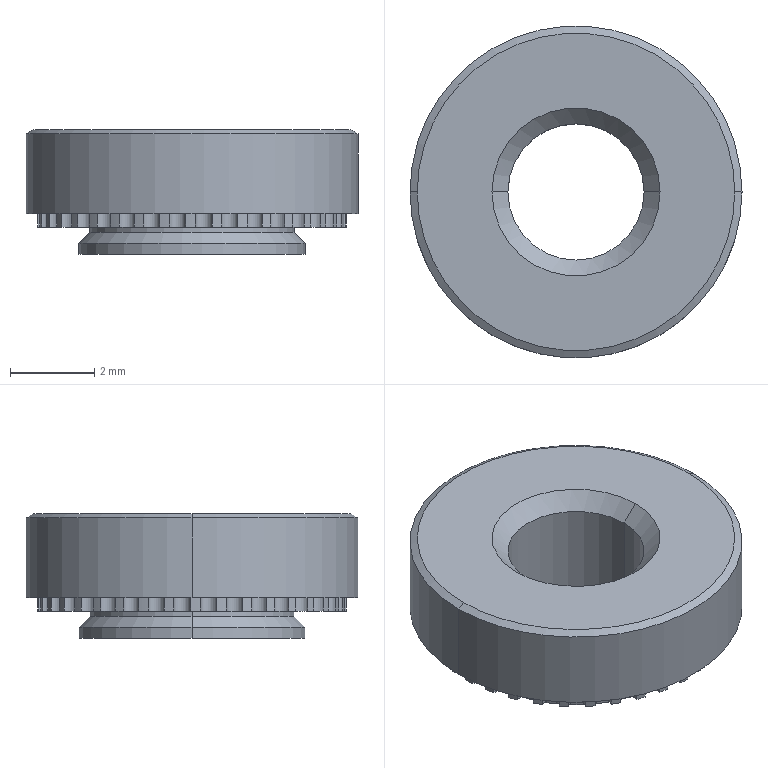Part | STEP file | M40001 | 1 solid | 94 faces | box 7.9 x 7.9 x 2.97 mm | volume 98.242 mm3 | cylinder 82 | cone 8 | plane 4 | commonest cylinder face diameters 0.4 x37 7.347 x37 3.242 x2 4.856 x2 5.38 x2 7.9 x2